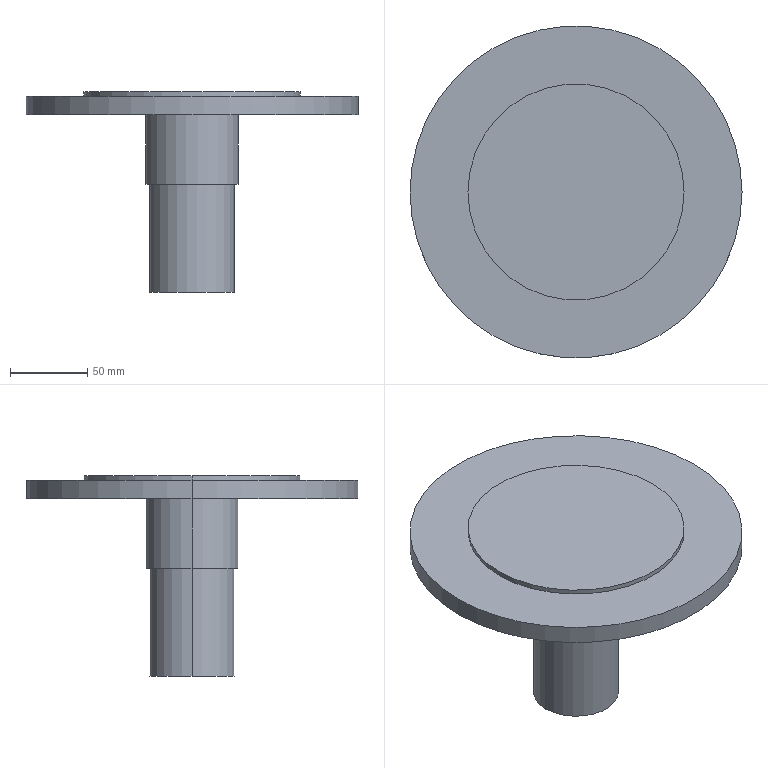Part | SolidWorks | features BaseBody 1 | 1 solid | 13 faces | box 215 x 215 x 130 mm | volume 775384 mm3 | cylinder 8 | plane 5 | commonest cylinder face diameters 55 x2 60 x2 140 x2 215 x2
STEP:
#1=CARTESIAN_POINT('',(30.,0.,-45.));
#2=VERTEX_POINT('',#1);
#3=CARTESIAN_POINT('',(-30.,0.,-45.));
#4=VERTEX_POINT('',#3);
#5=CARTESIAN_POINT('',(0.,0.,-45.));
#6=DIRECTION('',(0.,0.,1.));
#7=DIRECTION('',(1.,0.,0.));
#8=AXIS2_PLACEMENT_3D('',#5,#6,#7);
#9=CIRCLE('',#8,30.);
#10=EDGE_CURVE('',#2,#4,#9,.T.);
#11=ORIENTED_EDGE('',*,*,#10,.T.);
#12=CARTESIAN_POINT('',(-30.,0.,0.));
#13=VERTEX_POINT('',#12);
#14=CARTESIAN_POINT('',(-30.,0.,-45.));
#15=DIRECTION('',(0.,0.,1.));
#16=VECTOR('',#15,1000.);
#17=LINE('',#14,#16);
#18=EDGE_CURVE('',#4,#13,#17,.T.);
#19=ORIENTED_EDGE('',*,*,#18,.T.);
#20=CARTESIAN_POINT('',(30.,0.,0.));
#21=VERTEX_POINT('',#20);
#22=CARTESIAN_POINT('',(0.,0.,0.));
#23=DIRECTION('',(0.,0.,-1.));
#24=DIRECTION('',(1.,0.,0.));
#25=AXIS2_PLACEMENT_3D('',#22,#23,#24);
#26=CIRCLE('',#25,30.);
#27=EDGE_CURVE('',#13,#21,#26,.T.);
#28=ORIENTED_EDGE('',*,*,#27,.T.);
#29=CARTESIAN_POINT('',(30.,0.,-45.));
#30=DIRECTION('',(0.,0.,1.));
#31=VECTOR('',#30,1000.);
#32=LINE('',#29,#31);
#33=EDGE_CURVE('',#2,#21,#32,.T.);
#34=ORIENTED_EDGE('',*,*,#33,.F.);
#35=EDGE_LOOP('',(#11,#19,#28,#34));
#36=FACE_OUTER_BOUND('',#35,.T.);
#37=CARTESIAN_POINT('',(0.,0.,-45.));
#38=DIRECTION('',(0.,0.,1.));
#39=DIRECTION('',(1.,0.,0.));
#40=AXIS2_PLACEMENT_3D('',#37,#38,#39);
#41=CYLINDRICAL_SURFACE('',#40,30.);
#42=ADVANCED_FACE('',(#36),#41,.T.);
#43=CARTESIAN_POINT('',(-107.5,0.,12.));
#44=VERTEX_POINT('',#43);
#45=CARTESIAN_POINT('',(107.5,0.,12.));
#46=VERTEX_POINT('',#45);
#47=CARTESIAN_POINT('',(0.,0.,12.));
#48=DIRECTION('',(0.,0.,-1.));
#49=DIRECTION('',(-1.,0.,0.));
#50=AXIS2_PLACEMENT_3D('',#47,#48,#49);
#51=CIRCLE('',#50,107.5);
#52=EDGE_CURVE('',#44,#46,#51,.T.);
#53=ORIENTED_EDGE('',*,*,#52,.T.);
#54=CARTESIAN_POINT('',(107.5,0.,0.));
#55=VERTEX_POINT('',#54);
#56=CARTESIAN_POINT('',(107.5,0.,12.));
#57=DIRECTION('',(0.,0.,-1.));
#58=VECTOR('',#57,1000.);
#59=LINE('',#56,#58);
#60=EDGE_CURVE('',#46,#55,#59,.T.);
#61=ORIENTED_EDGE('',*,*,#60,.T.);
#62=CARTESIAN_POINT('',(-107.5,0.,0.));
#63=VERTEX_POINT('',#62);
#64=CARTESIAN_POINT('',(0.,0.,0.));
#65=DIRECTION('',(0.,0.,1.));
#66=DIRECTION('',(-1.,0.,0.));
#67=AXIS2_PLACEMENT_3D('',#64,#65,#66);
#68=CIRCLE('',#67,107.5);
#69=EDGE_CURVE('',#55,#63,#68,.T.);
#70=ORIENTED_EDGE('',*,*,#69,.T.);
#71=CARTESIAN_POINT('',(-107.5,0.,12.));
#72=DIRECTION('',(0.,0.,-1.));
#73=VECTOR('',#72,1000.);
#74=LINE('',#71,#73);
#75=EDGE_CURVE('',#44,#63,#74,.T.);
#76=ORIENTED_EDGE('',*,*,#75,.F.);
#77=EDGE_LOOP('',(#53,#61,#70,#76));
#78=FACE_OUTER_BOUND('',#77,.T.);
#79=CARTESIAN_POINT('',(0.,0.,12.));
#80=DIRECTION('',(0.,0.,-1.));
#81=DIRECTION('',(-1.,0.,0.));
#82=AXIS2_PLACEMENT_3D('',#79,#80,#81);
#83=CYLINDRICAL_SURFACE('',#82,107.5);
#84=ADVANCED_FACE('',(#78),#83,.T.);
#85=CARTESIAN_POINT('',(27.5,0.,-115.));
#86=VERTEX_POINT('',#85);
#87=CARTESIAN_POINT('',(-27.5,0.,-115.));
#88=VERTEX_POINT('',#87);
#89=CARTESIAN_POINT('',(0.,0.,-115.));
#90=DIRECTION('',(0.,0.,1.));
#91=DIRECTION('',(1.,0.,0.));
#92=AXIS2_PLACEMENT_3D('',#89,#90,#91);
#93=CIRCLE('',#92,27.5);
#94=EDGE_CURVE('',#86,#88,#93,.T.);
#95=ORIENTED_EDGE('',*,*,#94,.T.);
#96=CARTESIAN_POINT('',(-27.5,0.,-45.));
#97=VERTEX_POINT('',#96);
#98=CARTESIAN_POINT('',(-27.5,0.,-115.));
#99=DIRECTION('',(0.,0.,1.));
#100=VECTOR('',#99,1000.);
#101=LINE('',#98,#100);
#102=EDGE_CURVE('',#88,#97,#101,.T.);
#103=ORIENTED_EDGE('',*,*,#102,.T.);
#104=CARTESIAN_POINT('',(27.5,0.,-45.));
#105=VERTEX_POINT('',#104);
#106=CARTESIAN_POINT('',(0.,0.,-45.));
#107=DIRECTION('',(0.,0.,-1.));
#108=DIRECTION('',(1.,0.,0.));
#109=AXIS2_PLACEMENT_3D('',#106,#107,#108);
#110=CIRCLE('',#109,27.5);
#111=EDGE_CURVE('',#97,#105,#110,.T.);
#112=ORIENTED_EDGE('',*,*,#111,.T.);
#113=CARTESIAN_POINT('',(27.5,0.,-115.));
#114=DIRECTION('',(0.,0.,1.));
#115=VECTOR('',#114,1000.);
#116=LINE('',#113,#115);
#117=EDGE_CURVE('',#86,#105,#116,.T.);
#118=ORIENTED_EDGE('',*,*,#117,.F.);
#119=EDGE_LOOP('',(#95,#103,#112,#118));
#120=FACE_OUTER_BOUND('',#119,.T.);
#121=CARTESIAN_POINT('',(0.,0.,-115.));
#122=DIRECTION('',(0.,0.,1.));
#123=DIRECTION('',(1.,0.,0.));
#124=AXIS2_PLACEMENT_3D('',#121,#122,#123);
#125=CYLINDRICAL_SURFACE('',#124,27.5);
#126=ADVANCED_FACE('',(#120),#125,.T.);
#127=CARTESIAN_POINT('',(-70.,0.,15.));
#128=VERTEX_POINT('',#127);
#129=CARTESIAN_POINT('',(70.,0.,15.));
#130=VERTEX_POINT('',#129);
#131=CARTESIAN_POINT('',(0.,0.,15.));
#132=DIRECTION('',(0.,0.,-1.));
#133=DIRECTION('',(-1.,0.,0.));
#134=AXIS2_PLACEMENT_3D('',#131,#132,#133);
#135=CIRCLE('',#134,70.);
#136=EDGE_CURVE('',#128,#130,#135,.T.);
#137=ORIENTED_EDGE('',*,*,#136,.T.);
#138=CARTESIAN_POINT('',(70.,0.,12.));
#139=VERTEX_POINT('',#138);
#140=CARTESIAN_POINT('',(70.,0.,15.));
#141=DIRECTION('',(0.,0.,-1.));
#142=VECTOR('',#141,1000.);
#143=LINE('',#140,#142);
#144=EDGE_CURVE('',#130,#139,#143,.T.);
#145=ORIENTED_EDGE('',*,*,#144,.T.);
#146=CARTESIAN_POINT('',(-70.,0.,12.));
#147=VERTEX_POINT('',#146);
#148=CARTESIAN_POINT('',(0.,0.,12.));
#149=DIRECTION('',(0.,0.,-1.));
#150=DIRECTION('',(-1.,0.,0.));
#151=AXIS2_PLACEMENT_3D('',#148,#149,#150);
#152=CIRCLE('',#151,70.);
#153=EDGE_CURVE('',#147,#139,#152,.T.);
#154=ORIENTED_EDGE('',*,*,#153,.F.);
#155=CARTESIAN_POINT('',(-70.,0.,15.));
#156=DIRECTION('',(0.,0.,-1.));
#157=VECTOR('',#156,1000.);
#158=LINE('',#155,#157);
#159=EDGE_CURVE('',#128,#147,#158,.T.);
#160=ORIENTED_EDGE('',*,*,#159,.F.);
#161=EDGE_LOOP('',(#137,#145,#154,#160));
#162=FACE_OUTER_BOUND('',#161,.T.);
#163=CARTESIAN_POINT('',(0.,0.,15.));
#164=DIRECTION('',(0.,0.,-1.));
#165=DIRECTION('',(-1.,0.,0.));
#166=AXIS2_PLACEMENT_3D('',#163,#164,#165);
#167=CYLINDRICAL_SURFACE('',#166,70.);
#168=ADVANCED_FACE('',(#162),#167,.T.);
#169=CARTESIAN_POINT('',(0.,0.,0.));
#170=DIRECTION('',(0.,0.,-1.));
#171=DIRECTION('',(1.,0.,0.));
#172=AXIS2_PLACEMENT_3D('',#169,#170,#171);
#173=CIRCLE('',#172,30.);
#174=EDGE_CURVE('',#21,#13,#173,.T.);
#175=ORIENTED_EDGE('',*,*,#174,.F.);
#176=ORIENTED_EDGE('',*,*,#27,.F.);
#177=EDGE_LOOP('',(#175,#176));
#178=FACE_BOUND('',#177,.T.);
#179=CARTESIAN_POINT('',(0.,0.,0.));
#180=DIRECTION('',(0.,0.,1.));
#181=DIRECTION('',(-1.,0.,0.));
#182=AXIS2_PLACEMENT_3D('',#179,#180,#181);
#183=CIRCLE('',#182,107.5);
#184=EDGE_CURVE('',#63,#55,#183,.T.);
#185=ORIENTED_EDGE('',*,*,#184,.F.);
#186=ORIENTED_EDGE('',*,*,#69,.F.);
#187=EDGE_LOOP('',(#185,#186));
#188=FACE_OUTER_BOUND('',#187,.T.);
#189=CARTESIAN_POINT('',(0.,0.,0.));
#190=DIRECTION('',(0.,0.,1.));
#191=DIRECTION('',(1.,0.,0.));
#192=AXIS2_PLACEMENT_3D('',#189,#190,#191);
#193=PLANE('',#192);
#194=ADVANCED_FACE('',(#178,#188),#193,.F.);
#195=ORIENTED_EDGE('',*,*,#18,.F.);
#196=CARTESIAN_POINT('',(0.,0.,-45.));
#197=DIRECTION('',(0.,0.,1.));
#198=DIRECTION('',(1.,0.,0.));
#199=AXIS2_PLACEMENT_3D('',#196,#197,#198);
#200=CIRCLE('',#199,30.);
#201=EDGE_CURVE('',#4,#2,#200,.T.);
#202=ORIENTED_EDGE('',*,*,#201,.T.);
#203=ORIENTED_EDGE('',*,*,#33,.T.);
#204=ORIENTED_EDGE('',*,*,#174,.T.);
#205=EDGE_LOOP('',(#195,#202,#203,#204));
#206=FACE_OUTER_BOUND('',#205,.T.);
#207=CARTESIAN_POINT('',(0.,0.,-45.));
#208=DIRECTION('',(0.,0.,1.));
#209=DIRECTION('',(1.,0.,0.));
#210=AXIS2_PLACEMENT_3D('',#207,#208,#209);
#211=CYLINDRICAL_SURFACE('',#210,30.);
#212=ADVANCED_FACE('',(#206),#211,.T.);
#213=ORIENTED_EDGE('',*,*,#60,.F.);
#214=CARTESIAN_POINT('',(0.,0.,12.));
#215=DIRECTION('',(0.,0.,-1.));
#216=DIRECTION('',(-1.,0.,0.));
#217=AXIS2_PLACEMENT_3D('',#214,#215,#216);
#218=CIRCLE('',#217,107.5);
#219=EDGE_CURVE('',#46,#44,#218,.T.);
#220=ORIENTED_EDGE('',*,*,#219,.T.);
#221=ORIENTED_EDGE('',*,*,#75,.T.);
#222=ORIENTED_EDGE('',*,*,#184,.T.);
#223=EDGE_LOOP('',(#213,#220,#221,#222));
#224=FACE_OUTER_BOUND('',#223,.T.);
#225=CARTESIAN_POINT('',(0.,0.,12.));
#226=DIRECTION('',(0.,0.,-1.));
#227=DIRECTION('',(-1.,0.,0.));
#228=AXIS2_PLACEMENT_3D('',#225,#226,#227);
#229=CYLINDRICAL_SURFACE('',#228,107.5);
#230=ADVANCED_FACE('',(#224),#229,.T.);
#231=CARTESIAN_POINT('',(0.,0.,-45.));
#232=DIRECTION('',(0.,0.,-1.));
#233=DIRECTION('',(1.,0.,0.));
#234=AXIS2_PLACEMENT_3D('',#231,#232,#233);
#235=CIRCLE('',#234,27.5);
#236=EDGE_CURVE('',#105,#97,#235,.T.);
#237=ORIENTED_EDGE('',*,*,#236,.F.);
#238=ORIENTED_EDGE('',*,*,#111,.F.);
#239=EDGE_LOOP('',(#237,#238));
#240=FACE_BOUND('',#239,.T.);
#241=ORIENTED_EDGE('',*,*,#10,.F.);
#242=ORIENTED_EDGE('',*,*,#201,.F.);
#243=EDGE_LOOP('',(#241,#242));
#244=FACE_OUTER_BOUND('',#243,.T.);
#245=CARTESIAN_POINT('',(0.,0.,-45.));
#246=DIRECTION('',(0.,0.,1.));
#247=DIRECTION('',(1.,0.,0.));
#248=AXIS2_PLACEMENT_3D('',#245,#246,#247);
#249=PLANE('',#248);
#250=ADVANCED_FACE('',(#240,#244),#249,.F.);
#251=ORIENTED_EDGE('',*,*,#153,.T.);
#252=CARTESIAN_POINT('',(0.,0.,12.));
#253=DIRECTION('',(0.,0.,-1.));
#254=DIRECTION('',(-1.,0.,0.));
#255=AXIS2_PLACEMENT_3D('',#252,#253,#254);
#256=CIRCLE('',#255,70.);
#257=EDGE_CURVE('',#139,#147,#256,.T.);
#258=ORIENTED_EDGE('',*,*,#257,.T.);
#259=EDGE_LOOP('',(#251,#258));
#260=FACE_BOUND('',#259,.T.);
#261=ORIENTED_EDGE('',*,*,#52,.F.);
#262=ORIENTED_EDGE('',*,*,#219,.F.);
#263=EDGE_LOOP('',(#261,#262));
#264=FACE_OUTER_BOUND('',#263,.T.);
#265=CARTESIAN_POINT('',(0.,0.,12.));
#266=DIRECTION('',(0.,0.,1.));
#267=DIRECTION('',(1.,0.,0.));
#268=AXIS2_PLACEMENT_3D('',#265,#266,#267);
#269=PLANE('',#268);
#270=ADVANCED_FACE('',(#260,#264),#269,.T.);
#271=ORIENTED_EDGE('',*,*,#102,.F.);
#272=CARTESIAN_POINT('',(0.,0.,-115.));
#273=DIRECTION('',(0.,0.,1.));
#274=DIRECTION('',(1.,0.,0.));
#275=AXIS2_PLACEMENT_3D('',#272,#273,#274);
#276=CIRCLE('',#275,27.5);
#277=EDGE_CURVE('',#88,#86,#276,.T.);
#278=ORIENTED_EDGE('',*,*,#277,.T.);
#279=ORIENTED_EDGE('',*,*,#117,.T.);
#280=ORIENTED_EDGE('',*,*,#236,.T.);
#281=EDGE_LOOP('',(#271,#278,#279,#280));
#282=FACE_OUTER_BOUND('',#281,.T.);
#283=CARTESIAN_POINT('',(0.,0.,-115.));
#284=DIRECTION('',(0.,0.,1.));
#285=DIRECTION('',(1.,0.,0.));
#286=AXIS2_PLACEMENT_3D('',#283,#284,#285);
#287=CYLINDRICAL_SURFACE('',#286,27.5);
#288=ADVANCED_FACE('',(#282),#287,.T.);
#289=ORIENTED_EDGE('',*,*,#144,.F.);
#290=CARTESIAN_POINT('',(0.,0.,15.));
#291=DIRECTION('',(0.,0.,-1.));
#292=DIRECTION('',(-1.,0.,0.));
#293=AXIS2_PLACEMENT_3D('',#290,#291,#292);
#294=CIRCLE('',#293,70.);
#295=EDGE_CURVE('',#130,#128,#294,.T.);
#296=ORIENTED_EDGE('',*,*,#295,.T.);
#297=ORIENTED_EDGE('',*,*,#159,.T.);
#298=ORIENTED_EDGE('',*,*,#257,.F.);
#299=EDGE_LOOP('',(#289,#296,#297,#298));
#300=FACE_OUTER_BOUND('',#299,.T.);
#301=CARTESIAN_POINT('',(0.,0.,15.));
#302=DIRECTION('',(0.,0.,-1.));
#303=DIRECTION('',(-1.,0.,0.));
#304=AXIS2_PLACEMENT_3D('',#301,#302,#303);
#305=CYLINDRICAL_SURFACE('',#304,70.);
#306=ADVANCED_FACE('',(#300),#305,.T.);
#307=ORIENTED_EDGE('',*,*,#94,.F.);
#308=ORIENTED_EDGE('',*,*,#277,.F.);
#309=EDGE_LOOP('',(#307,#308));
#310=FACE_OUTER_BOUND('',#309,.T.);
#311=CARTESIAN_POINT('',(0.,0.,-115.));
#312=DIRECTION('',(0.,0.,1.));
#313=DIRECTION('',(1.,0.,0.));
#314=AXIS2_PLACEMENT_3D('',#311,#312,#313);
#315=PLANE('',#314);
#316=ADVANCED_FACE('',(#310),#315,.F.);
#317=ORIENTED_EDGE('',*,*,#136,.F.);
#318=ORIENTED_EDGE('',*,*,#295,.F.);
#319=EDGE_LOOP('',(#317,#318));
#320=FACE_OUTER_BOUND('',#319,.T.);
#321=CARTESIAN_POINT('',(0.,0.,15.));
#322=DIRECTION('',(0.,0.,1.));
#323=DIRECTION('',(1.,0.,0.));
#324=AXIS2_PLACEMENT_3D('',#321,#322,#323);
#325=PLANE('',#324);
#326=ADVANCED_FACE('',(#320),#325,.T.);
#327=CLOSED_SHELL('',(#42,#84,#126,#168,#194,#212,#230,#250,#270,#288,#306,#316,#326));
#328=MANIFOLD_SOLID_BREP('',#327);
#329=CARTESIAN_POINT('',(0.,0.,0.));
#330=DIRECTION('',(0.,0.,1.));
#331=DIRECTION('',(1.,0.,0.));
#332=AXIS2_PLACEMENT_3D('',#329,#330,#331);
#333=(LENGTH_UNIT()NAMED_UNIT(*)SI_UNIT(.MILLI.,.METRE.));
#334=UNCERTAINTY_MEASURE_WITH_UNIT(LENGTH_MEASURE(0.00001),#333,'','');
#335=(NAMED_UNIT(*)PLANE_ANGLE_UNIT()SI_UNIT($,.RADIAN.));
#336=(NAMED_UNIT(*)SI_UNIT($,.STERADIAN.)SOLID_ANGLE_UNIT());
#337=(GEOMETRIC_REPRESENTATION_CONTEXT(3)GLOBAL_UNCERTAINTY_ASSIGNED_CONTEXT((#334))GLOBAL_UNIT_ASSIGNED_CONTEXT((#333,#335,#336))REPRESENTATION_CONTEXT('',''));
#338=ADVANCED_BREP_SHAPE_REPRESENTATION('',(#328,#332),#337);